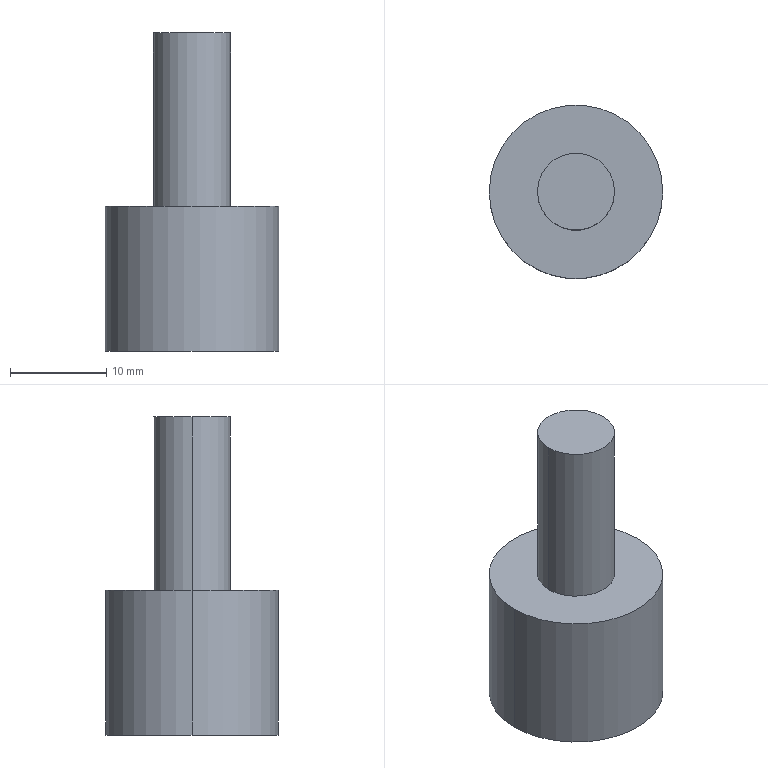Part | 1 solid | 10 faces | box 18 x 18 x 33 mm | volume 3541 mm3 | cylinder 4 | plane 4 | cone 2 | commonest cylinder face diameters 8 x2 18 x2
STEP:
#1=CARTESIAN_POINT('',(-3.405,0.,10.));
#2=VERTEX_POINT('',#1);
#3=CARTESIAN_POINT('',(3.405,0.,10.));
#4=VERTEX_POINT('',#3);
#5=CARTESIAN_POINT('',(0.,0.,10.));
#6=DIRECTION('',(0.,0.,1.));
#7=DIRECTION('',(1.,0.,0.));
#8=AXIS2_PLACEMENT_3D('',#5,#6,#7);
#9=CIRCLE('',#8,3.405);
#10=EDGE_CURVE('',#2,#4,#9,.T.);
#11=ORIENTED_EDGE('',*,*,#10,.T.);
#12=CARTESIAN_POINT('',(8.5,0.,0.));
#13=VERTEX_POINT('',#12);
#14=CARTESIAN_POINT('',(3.405,0.,10.));
#15=DIRECTION('',(0.454,0.,-0.891));
#16=VECTOR('',#15,1000.);
#17=LINE('',#14,#16);
#18=EDGE_CURVE('',#4,#13,#17,.T.);
#19=ORIENTED_EDGE('',*,*,#18,.T.);
#20=CARTESIAN_POINT('',(-8.5,0.,0.));
#21=VERTEX_POINT('',#20);
#22=CARTESIAN_POINT('',(0.,0.,0.));
#23=DIRECTION('',(0.,0.,1.));
#24=DIRECTION('',(1.,0.,0.));
#25=AXIS2_PLACEMENT_3D('',#22,#23,#24);
#26=CIRCLE('',#25,8.5);
#27=EDGE_CURVE('',#21,#13,#26,.T.);
#28=ORIENTED_EDGE('',*,*,#27,.F.);
#29=CARTESIAN_POINT('',(-3.405,0.,10.));
#30=DIRECTION('',(-0.454,0.,-0.891));
#31=VECTOR('',#30,1000.);
#32=LINE('',#29,#31);
#33=EDGE_CURVE('',#2,#21,#32,.T.);
#34=ORIENTED_EDGE('',*,*,#33,.F.);
#35=EDGE_LOOP('',(#11,#19,#28,#34));
#36=FACE_OUTER_BOUND('',#35,.T.);
#37=CARTESIAN_POINT('',(0.,0.,10.));
#38=DIRECTION('',(0.,0.,-1.));
#39=DIRECTION('',(-1.,0.,0.));
#40=AXIS2_PLACEMENT_3D('',#37,#38,#39);
#41=CONICAL_SURFACE('',#40,3.405,0.4712);
#42=ADVANCED_FACE('',(#36),#41,.F.);
#43=CARTESIAN_POINT('',(4.,0.,33.));
#44=VERTEX_POINT('',#43);
#45=CARTESIAN_POINT('',(-4.,0.,33.));
#46=VERTEX_POINT('',#45);
#47=CARTESIAN_POINT('',(0.,0.,33.));
#48=DIRECTION('',(0.,0.,1.));
#49=DIRECTION('',(1.,0.,0.));
#50=AXIS2_PLACEMENT_3D('',#47,#48,#49);
#51=CIRCLE('',#50,4.);
#52=EDGE_CURVE('',#44,#46,#51,.T.);
#53=ORIENTED_EDGE('',*,*,#52,.F.);
#54=CARTESIAN_POINT('',(4.,0.,15.));
#55=VERTEX_POINT('',#54);
#56=CARTESIAN_POINT('',(4.,0.,33.));
#57=DIRECTION('',(0.,0.,-1.));
#58=VECTOR('',#57,1000.);
#59=LINE('',#56,#58);
#60=EDGE_CURVE('',#44,#55,#59,.T.);
#61=ORIENTED_EDGE('',*,*,#60,.T.);
#62=CARTESIAN_POINT('',(-4.,0.,15.));
#63=VERTEX_POINT('',#62);
#64=CARTESIAN_POINT('',(0.,0.,15.));
#65=DIRECTION('',(0.,0.,1.));
#66=DIRECTION('',(1.,0.,0.));
#67=AXIS2_PLACEMENT_3D('',#64,#65,#66);
#68=CIRCLE('',#67,4.);
#69=EDGE_CURVE('',#55,#63,#68,.T.);
#70=ORIENTED_EDGE('',*,*,#69,.T.);
#71=CARTESIAN_POINT('',(-4.,0.,33.));
#72=DIRECTION('',(0.,0.,-1.));
#73=VECTOR('',#72,1000.);
#74=LINE('',#71,#73);
#75=EDGE_CURVE('',#46,#63,#74,.T.);
#76=ORIENTED_EDGE('',*,*,#75,.F.);
#77=EDGE_LOOP('',(#53,#61,#70,#76));
#78=FACE_OUTER_BOUND('',#77,.T.);
#79=CARTESIAN_POINT('',(0.,0.,33.));
#80=DIRECTION('',(0.,0.,-1.));
#81=DIRECTION('',(-1.,0.,0.));
#82=AXIS2_PLACEMENT_3D('',#79,#80,#81);
#83=CYLINDRICAL_SURFACE('',#82,4.);
#84=ADVANCED_FACE('',(#78),#83,.T.);
#85=CARTESIAN_POINT('',(9.,0.,15.));
#86=VERTEX_POINT('',#85);
#87=CARTESIAN_POINT('',(-9.,0.,15.));
#88=VERTEX_POINT('',#87);
#89=CARTESIAN_POINT('',(0.,0.,15.));
#90=DIRECTION('',(0.,0.,1.));
#91=DIRECTION('',(1.,0.,0.));
#92=AXIS2_PLACEMENT_3D('',#89,#90,#91);
#93=CIRCLE('',#92,9.);
#94=EDGE_CURVE('',#86,#88,#93,.T.);
#95=ORIENTED_EDGE('',*,*,#94,.F.);
#96=CARTESIAN_POINT('',(9.,0.,0.));
#97=VERTEX_POINT('',#96);
#98=CARTESIAN_POINT('',(9.,0.,15.));
#99=DIRECTION('',(0.,0.,-1.));
#100=VECTOR('',#99,1000.);
#101=LINE('',#98,#100);
#102=EDGE_CURVE('',#86,#97,#101,.T.);
#103=ORIENTED_EDGE('',*,*,#102,.T.);
#104=CARTESIAN_POINT('',(-9.,0.,0.));
#105=VERTEX_POINT('',#104);
#106=CARTESIAN_POINT('',(0.,0.,0.));
#107=DIRECTION('',(0.,0.,1.));
#108=DIRECTION('',(1.,0.,0.));
#109=AXIS2_PLACEMENT_3D('',#106,#107,#108);
#110=CIRCLE('',#109,9.);
#111=EDGE_CURVE('',#97,#105,#110,.T.);
#112=ORIENTED_EDGE('',*,*,#111,.T.);
#113=CARTESIAN_POINT('',(-9.,0.,15.));
#114=DIRECTION('',(0.,0.,-1.));
#115=VECTOR('',#114,1000.);
#116=LINE('',#113,#115);
#117=EDGE_CURVE('',#88,#105,#116,.T.);
#118=ORIENTED_EDGE('',*,*,#117,.F.);
#119=EDGE_LOOP('',(#95,#103,#112,#118));
#120=FACE_OUTER_BOUND('',#119,.T.);
#121=CARTESIAN_POINT('',(0.,0.,15.));
#122=DIRECTION('',(0.,0.,-1.));
#123=DIRECTION('',(-1.,0.,0.));
#124=AXIS2_PLACEMENT_3D('',#121,#122,#123);
#125=CYLINDRICAL_SURFACE('',#124,9.);
#126=ADVANCED_FACE('',(#120),#125,.T.);
#127=CARTESIAN_POINT('',(0.,0.,15.));
#128=DIRECTION('',(0.,0.,1.));
#129=DIRECTION('',(1.,0.,0.));
#130=AXIS2_PLACEMENT_3D('',#127,#128,#129);
#131=CIRCLE('',#130,9.);
#132=EDGE_CURVE('',#88,#86,#131,.T.);
#133=ORIENTED_EDGE('',*,*,#132,.T.);
#134=ORIENTED_EDGE('',*,*,#94,.T.);
#135=EDGE_LOOP('',(#133,#134));
#136=FACE_OUTER_BOUND('',#135,.T.);
#137=CARTESIAN_POINT('',(0.,0.,15.));
#138=DIRECTION('',(0.,0.,1.));
#139=DIRECTION('',(1.,0.,0.));
#140=AXIS2_PLACEMENT_3D('',#137,#138,#139);
#141=CIRCLE('',#140,4.);
#142=EDGE_CURVE('',#63,#55,#141,.T.);
#143=ORIENTED_EDGE('',*,*,#142,.F.);
#144=ORIENTED_EDGE('',*,*,#69,.F.);
#145=EDGE_LOOP('',(#143,#144));
#146=FACE_BOUND('',#145,.T.);
#147=CARTESIAN_POINT('',(0.,0.,15.));
#148=DIRECTION('',(0.,0.,1.));
#149=DIRECTION('',(1.,0.,0.));
#150=AXIS2_PLACEMENT_3D('',#147,#148,#149);
#151=PLANE('',#150);
#152=ADVANCED_FACE('',(#136,#146),#151,.T.);
#153=ORIENTED_EDGE('',*,*,#102,.F.);
#154=ORIENTED_EDGE('',*,*,#132,.F.);
#155=ORIENTED_EDGE('',*,*,#117,.T.);
#156=CARTESIAN_POINT('',(0.,0.,0.));
#157=DIRECTION('',(0.,0.,1.));
#158=DIRECTION('',(1.,0.,0.));
#159=AXIS2_PLACEMENT_3D('',#156,#157,#158);
#160=CIRCLE('',#159,9.);
#161=EDGE_CURVE('',#105,#97,#160,.T.);
#162=ORIENTED_EDGE('',*,*,#161,.T.);
#163=EDGE_LOOP('',(#153,#154,#155,#162));
#164=FACE_OUTER_BOUND('',#163,.T.);
#165=CARTESIAN_POINT('',(0.,0.,15.));
#166=DIRECTION('',(0.,0.,-1.));
#167=DIRECTION('',(-1.,0.,0.));
#168=AXIS2_PLACEMENT_3D('',#165,#166,#167);
#169=CYLINDRICAL_SURFACE('',#168,9.);
#170=ADVANCED_FACE('',(#164),#169,.T.);
#171=ORIENTED_EDGE('',*,*,#27,.T.);
#172=CARTESIAN_POINT('',(0.,0.,0.));
#173=DIRECTION('',(0.,0.,1.));
#174=DIRECTION('',(1.,0.,0.));
#175=AXIS2_PLACEMENT_3D('',#172,#173,#174);
#176=CIRCLE('',#175,8.5);
#177=EDGE_CURVE('',#13,#21,#176,.T.);
#178=ORIENTED_EDGE('',*,*,#177,.T.);
#179=EDGE_LOOP('',(#171,#178));
#180=FACE_BOUND('',#179,.T.);
#181=ORIENTED_EDGE('',*,*,#161,.F.);
#182=ORIENTED_EDGE('',*,*,#111,.F.);
#183=EDGE_LOOP('',(#181,#182));
#184=FACE_OUTER_BOUND('',#183,.T.);
#185=CARTESIAN_POINT('',(0.,0.,0.));
#186=DIRECTION('',(0.,0.,1.));
#187=DIRECTION('',(1.,0.,0.));
#188=AXIS2_PLACEMENT_3D('',#185,#186,#187);
#189=PLANE('',#188);
#190=ADVANCED_FACE('',(#180,#184),#189,.F.);
#191=ORIENTED_EDGE('',*,*,#60,.F.);
#192=CARTESIAN_POINT('',(0.,0.,33.));
#193=DIRECTION('',(0.,0.,1.));
#194=DIRECTION('',(1.,0.,0.));
#195=AXIS2_PLACEMENT_3D('',#192,#193,#194);
#196=CIRCLE('',#195,4.);
#197=EDGE_CURVE('',#46,#44,#196,.T.);
#198=ORIENTED_EDGE('',*,*,#197,.F.);
#199=ORIENTED_EDGE('',*,*,#75,.T.);
#200=ORIENTED_EDGE('',*,*,#142,.T.);
#201=EDGE_LOOP('',(#191,#198,#199,#200));
#202=FACE_OUTER_BOUND('',#201,.T.);
#203=CARTESIAN_POINT('',(0.,0.,33.));
#204=DIRECTION('',(0.,0.,-1.));
#205=DIRECTION('',(-1.,0.,0.));
#206=AXIS2_PLACEMENT_3D('',#203,#204,#205);
#207=CYLINDRICAL_SURFACE('',#206,4.);
#208=ADVANCED_FACE('',(#202),#207,.T.);
#209=ORIENTED_EDGE('',*,*,#197,.T.);
#210=ORIENTED_EDGE('',*,*,#52,.T.);
#211=EDGE_LOOP('',(#209,#210));
#212=FACE_OUTER_BOUND('',#211,.T.);
#213=CARTESIAN_POINT('',(0.,0.,33.));
#214=DIRECTION('',(0.,0.,1.));
#215=DIRECTION('',(1.,0.,0.));
#216=AXIS2_PLACEMENT_3D('',#213,#214,#215);
#217=PLANE('',#216);
#218=ADVANCED_FACE('',(#212),#217,.T.);
#219=ORIENTED_EDGE('',*,*,#10,.F.);
#220=CARTESIAN_POINT('',(0.,0.,10.));
#221=DIRECTION('',(0.,0.,1.));
#222=DIRECTION('',(1.,0.,0.));
#223=AXIS2_PLACEMENT_3D('',#220,#221,#222);
#224=CIRCLE('',#223,3.405);
#225=EDGE_CURVE('',#4,#2,#224,.T.);
#226=ORIENTED_EDGE('',*,*,#225,.F.);
#227=EDGE_LOOP('',(#219,#226));
#228=FACE_OUTER_BOUND('',#227,.T.);
#229=CARTESIAN_POINT('',(3.405,0.,10.));
#230=DIRECTION('',(0.,0.,1.));
#231=DIRECTION('',(1.,0.,0.));
#232=AXIS2_PLACEMENT_3D('',#229,#230,#231);
#233=PLANE('',#232);
#234=ADVANCED_FACE('',(#228),#233,.F.);
#235=ORIENTED_EDGE('',*,*,#18,.F.);
#236=ORIENTED_EDGE('',*,*,#225,.T.);
#237=ORIENTED_EDGE('',*,*,#33,.T.);
#238=ORIENTED_EDGE('',*,*,#177,.F.);
#239=EDGE_LOOP('',(#235,#236,#237,#238));
#240=FACE_OUTER_BOUND('',#239,.T.);
#241=CARTESIAN_POINT('',(0.,0.,10.));
#242=DIRECTION('',(0.,0.,-1.));
#243=DIRECTION('',(-1.,0.,0.));
#244=AXIS2_PLACEMENT_3D('',#241,#242,#243);
#245=CONICAL_SURFACE('',#244,3.405,0.4712);
#246=ADVANCED_FACE('',(#240),#245,.F.);
#247=CLOSED_SHELL('',(#42,#84,#126,#152,#170,#190,#208,#218,#234,#246));
#248=MANIFOLD_SOLID_BREP('',#247);
#249=CARTESIAN_POINT('',(0.,0.,0.));
#250=DIRECTION('',(0.,0.,1.));
#251=DIRECTION('',(1.,0.,0.));
#252=AXIS2_PLACEMENT_3D('',#249,#250,#251);
#253=(LENGTH_UNIT()NAMED_UNIT(*)SI_UNIT(.MILLI.,.METRE.));
#254=UNCERTAINTY_MEASURE_WITH_UNIT(LENGTH_MEASURE(0.00001),#253,'','');
#255=(NAMED_UNIT(*)PLANE_ANGLE_UNIT()SI_UNIT($,.RADIAN.));
#256=(NAMED_UNIT(*)SI_UNIT($,.STERADIAN.)SOLID_ANGLE_UNIT());
#257=(GEOMETRIC_REPRESENTATION_CONTEXT(3)GLOBAL_UNCERTAINTY_ASSIGNED_CONTEXT((#254))GLOBAL_UNIT_ASSIGNED_CONTEXT((#253,#255,#256))REPRESENTATION_CONTEXT('',''));
#258=ADVANCED_BREP_SHAPE_REPRESENTATION('',(#248,#252),#257);